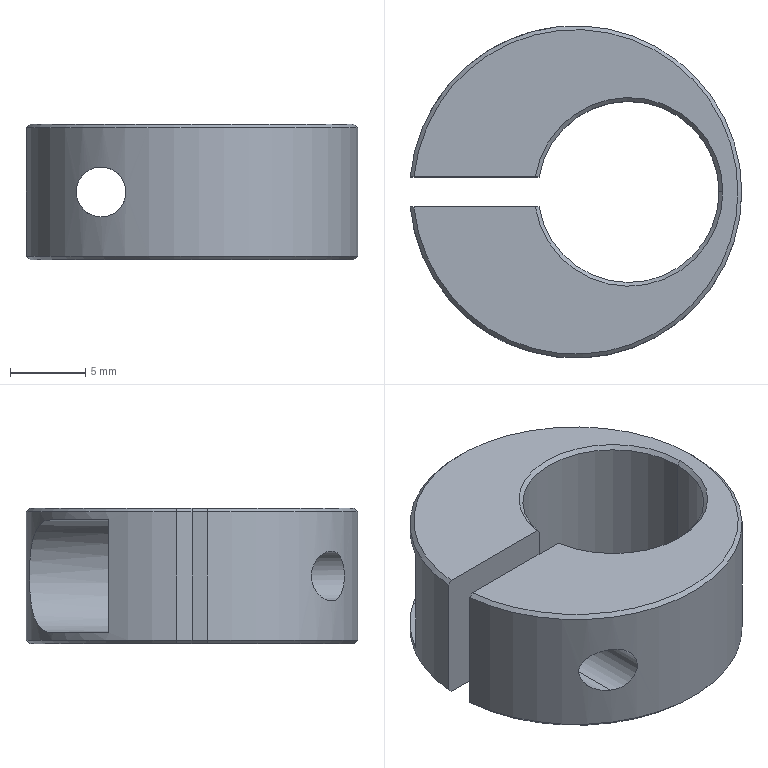Part | NX | features BREP 1 | 1 solid | 21 faces | box 21.954 x 22 x 9 mm | volume 1945 mm3 | cylinder 8 | plane 7 | cone 6 | commonest cylinder face diameters 3.3 x2 4.5 x2 12 x2 7.5 x1 22 x1
STEP:
#1=CARTESIAN_POINT('',(9.5,0.,8.75));
#2=VERTEX_POINT('',#1);
#3=CARTESIAN_POINT('',(9.75,0.,9.));
#4=VERTEX_POINT('',#3);
#5=CARTESIAN_POINT('',(9.5,0.,8.75));
#6=DIRECTION('',(0.7071,0.,0.7071));
#7=VECTOR('',#6,1000.);
#8=LINE('',#5,#7);
#9=EDGE_CURVE('',#2,#4,#8,.T.);
#10=ORIENTED_EDGE('',*,*,#9,.F.);
#11=CARTESIAN_POINT('',(-2.416,-1.,8.75));
#12=VERTEX_POINT('',#11);
#13=CARTESIAN_POINT('',(3.5,0.,8.75));
#14=DIRECTION('',(0.,0.,1.));
#15=DIRECTION('',(1.,0.,0.));
#16=AXIS2_PLACEMENT_3D('',#13,#14,#15);
#17=CIRCLE('',#16,6.);
#18=EDGE_CURVE('',#12,#2,#17,.T.);
#19=ORIENTED_EDGE('',*,*,#18,.F.);
#20=CARTESIAN_POINT('',(-2.669,-1.,9.));
#21=VERTEX_POINT('',#20);
#22=CARTESIAN_POINT('',(-2.669,-1.,9.));
#23=CARTESIAN_POINT('',(-2.585,-1.,8.917));
#24=CARTESIAN_POINT('',(-2.501,-1.,8.833));
#25=CARTESIAN_POINT('',(-2.416,-1.,8.75));
#26=B_SPLINE_CURVE_WITH_KNOTS('',3,(#22,#23,#24,#25),.UNSPECIFIED.,.F.,.F.,(4,4),(0.,0.000356),.UNSPECIFIED.);
#27=EDGE_CURVE('',#21,#12,#26,.T.);
#28=ORIENTED_EDGE('',*,*,#27,.F.);
#29=CARTESIAN_POINT('',(3.5,0.,9.));
#30=DIRECTION('',(0.,0.,-1.));
#31=DIRECTION('',(1.,0.,0.));
#32=AXIS2_PLACEMENT_3D('',#29,#30,#31);
#33=CIRCLE('',#32,6.25);
#34=EDGE_CURVE('',#4,#21,#33,.T.);
#35=ORIENTED_EDGE('',*,*,#34,.F.);
#36=EDGE_LOOP('',(#10,#19,#28,#35));
#37=FACE_BOUND('',#36,.T.);
#38=CARTESIAN_POINT('',(3.5,0.,8.75));
#39=DIRECTION('',(0.,0.,1.));
#40=DIRECTION('',(1.,0.,0.));
#41=AXIS2_PLACEMENT_3D('',#38,#39,#40);
#42=CONICAL_SURFACE('',#41,6.,0.7854);
#43=ADVANCED_FACE('',(#37),#42,.F.);
#44=CARTESIAN_POINT('',(-10.954,-1.,8.75));
#45=VERTEX_POINT('',#44);
#46=CARTESIAN_POINT('',(-10.703,-1.,9.));
#47=VERTEX_POINT('',#46);
#48=CARTESIAN_POINT('',(-10.954,-1.,8.75));
#49=CARTESIAN_POINT('',(-10.871,-1.,8.833));
#50=CARTESIAN_POINT('',(-10.787,-1.,8.917));
#51=CARTESIAN_POINT('',(-10.703,-1.,9.));
#52=B_SPLINE_CURVE_WITH_KNOTS('',3,(#48,#49,#50,#51),.UNSPECIFIED.,.F.,.F.,(4,4),(0.,0.0003543),.UNSPECIFIED.);
#53=EDGE_CURVE('',#45,#47,#52,.T.);
#54=ORIENTED_EDGE('',*,*,#53,.F.);
#55=CARTESIAN_POINT('',(-10.954,1.,8.75));
#56=VERTEX_POINT('',#55);
#57=CARTESIAN_POINT('',(0.,0.,8.75));
#58=DIRECTION('',(0.,0.,-1.));
#59=DIRECTION('',(1.,0.,0.));
#60=AXIS2_PLACEMENT_3D('',#57,#58,#59);
#61=CIRCLE('',#60,11.);
#62=EDGE_CURVE('',#56,#45,#61,.T.);
#63=ORIENTED_EDGE('',*,*,#62,.F.);
#64=CARTESIAN_POINT('',(-10.703,1.,9.));
#65=VERTEX_POINT('',#64);
#66=CARTESIAN_POINT('',(-10.703,1.,9.));
#67=CARTESIAN_POINT('',(-10.787,1.,8.917));
#68=CARTESIAN_POINT('',(-10.871,1.,8.833));
#69=CARTESIAN_POINT('',(-10.954,1.,8.75));
#70=B_SPLINE_CURVE_WITH_KNOTS('',3,(#66,#67,#68,#69),.UNSPECIFIED.,.F.,.F.,(4,4),(0.,0.0003543),.UNSPECIFIED.);
#71=EDGE_CURVE('',#65,#56,#70,.T.);
#72=ORIENTED_EDGE('',*,*,#71,.F.);
#73=CARTESIAN_POINT('',(0.,0.,9.));
#74=DIRECTION('',(0.,0.,1.));
#75=DIRECTION('',(1.,0.,0.));
#76=AXIS2_PLACEMENT_3D('',#73,#74,#75);
#77=CIRCLE('',#76,10.75);
#78=EDGE_CURVE('',#47,#65,#77,.T.);
#79=ORIENTED_EDGE('',*,*,#78,.F.);
#80=EDGE_LOOP('',(#54,#63,#72,#79));
#81=FACE_BOUND('',#80,.T.);
#82=CARTESIAN_POINT('',(0.,0.,9.));
#83=DIRECTION('',(0.,0.,-1.));
#84=DIRECTION('',(-1.,0.,0.));
#85=AXIS2_PLACEMENT_3D('',#82,#83,#84);
#86=CONICAL_SURFACE('',#85,10.75,0.7854);
#87=ADVANCED_FACE('',(#81),#86,.T.);
#88=CARTESIAN_POINT('',(-2.669,1.,0.));
#89=VERTEX_POINT('',#88);
#90=CARTESIAN_POINT('',(-2.416,1.,0.25));
#91=VERTEX_POINT('',#90);
#92=CARTESIAN_POINT('',(-2.669,1.,0.));
#93=CARTESIAN_POINT('',(-2.585,1.,0.08336));
#94=CARTESIAN_POINT('',(-2.501,1.,0.1667));
#95=CARTESIAN_POINT('',(-2.416,1.,0.25));
#96=B_SPLINE_CURVE_WITH_KNOTS('',3,(#92,#93,#94,#95),.UNSPECIFIED.,.F.,.F.,(4,4),(0.,0.000356),.UNSPECIFIED.);
#97=EDGE_CURVE('',#89,#91,#96,.T.);
#98=ORIENTED_EDGE('',*,*,#97,.F.);
#99=CARTESIAN_POINT('',(-2.669,-1.,0.));
#100=VERTEX_POINT('',#99);
#101=CARTESIAN_POINT('',(3.5,0.,0.));
#102=DIRECTION('',(0.,0.,1.));
#103=DIRECTION('',(1.,0.,0.));
#104=AXIS2_PLACEMENT_3D('',#101,#102,#103);
#105=CIRCLE('',#104,6.25);
#106=EDGE_CURVE('',#100,#89,#105,.T.);
#107=ORIENTED_EDGE('',*,*,#106,.F.);
#108=CARTESIAN_POINT('',(-2.416,-1.,0.25));
#109=VERTEX_POINT('',#108);
#110=CARTESIAN_POINT('',(-2.416,-1.,0.25));
#111=CARTESIAN_POINT('',(-2.501,-1.,0.1667));
#112=CARTESIAN_POINT('',(-2.585,-1.,0.08336));
#113=CARTESIAN_POINT('',(-2.669,-1.,0.));
#114=B_SPLINE_CURVE_WITH_KNOTS('',3,(#110,#111,#112,#113),.UNSPECIFIED.,.F.,.F.,(4,4),(0.,0.000356),.UNSPECIFIED.);
#115=EDGE_CURVE('',#109,#100,#114,.T.);
#116=ORIENTED_EDGE('',*,*,#115,.F.);
#117=CARTESIAN_POINT('',(9.5,0.,0.25));
#118=VERTEX_POINT('',#117);
#119=CARTESIAN_POINT('',(3.5,0.,0.25));
#120=DIRECTION('',(0.,0.,-1.));
#121=DIRECTION('',(1.,0.,0.));
#122=AXIS2_PLACEMENT_3D('',#119,#120,#121);
#123=CIRCLE('',#122,6.);
#124=EDGE_CURVE('',#118,#109,#123,.T.);
#125=ORIENTED_EDGE('',*,*,#124,.F.);
#126=CARTESIAN_POINT('',(3.5,0.,0.25));
#127=DIRECTION('',(0.,0.,-1.));
#128=DIRECTION('',(1.,0.,0.));
#129=AXIS2_PLACEMENT_3D('',#126,#127,#128);
#130=CIRCLE('',#129,6.);
#131=EDGE_CURVE('',#91,#118,#130,.T.);
#132=ORIENTED_EDGE('',*,*,#131,.F.);
#133=EDGE_LOOP('',(#98,#107,#116,#125,#132));
#134=FACE_BOUND('',#133,.T.);
#135=CARTESIAN_POINT('',(3.5,0.,0.25));
#136=DIRECTION('',(0.,0.,-1.));
#137=DIRECTION('',(-1.,0.,0.));
#138=AXIS2_PLACEMENT_3D('',#135,#136,#137);
#139=CONICAL_SURFACE('',#138,6.,0.7854);
#140=ADVANCED_FACE('',(#134),#139,.F.);
#141=CARTESIAN_POINT('',(10.75,0.,0.));
#142=VERTEX_POINT('',#141);
#143=CARTESIAN_POINT('',(11.,0.,0.25));
#144=VERTEX_POINT('',#143);
#145=CARTESIAN_POINT('',(11.,0.,0.25));
#146=DIRECTION('',(0.7071,0.,0.7071));
#147=VECTOR('',#146,1000.);
#148=LINE('',#145,#147);
#149=EDGE_CURVE('',#142,#144,#148,.T.);
#150=ORIENTED_EDGE('',*,*,#149,.F.);
#151=CARTESIAN_POINT('',(-10.703,1.,0.));
#152=VERTEX_POINT('',#151);
#153=CARTESIAN_POINT('',(0.,0.,0.));
#154=DIRECTION('',(0.,0.,-1.));
#155=DIRECTION('',(1.,0.,0.));
#156=AXIS2_PLACEMENT_3D('',#153,#154,#155);
#157=CIRCLE('',#156,10.75);
#158=EDGE_CURVE('',#152,#142,#157,.T.);
#159=ORIENTED_EDGE('',*,*,#158,.F.);
#160=CARTESIAN_POINT('',(-10.954,1.,0.25));
#161=VERTEX_POINT('',#160);
#162=CARTESIAN_POINT('',(-10.954,1.,0.25));
#163=CARTESIAN_POINT('',(-10.871,1.,0.1667));
#164=CARTESIAN_POINT('',(-10.787,1.,0.08333));
#165=CARTESIAN_POINT('',(-10.703,1.,0.));
#166=B_SPLINE_CURVE_WITH_KNOTS('',3,(#162,#163,#164,#165),.UNSPECIFIED.,.F.,.F.,(4,4),(0.,0.0003543),.UNSPECIFIED.);
#167=EDGE_CURVE('',#161,#152,#166,.T.);
#168=ORIENTED_EDGE('',*,*,#167,.F.);
#169=CARTESIAN_POINT('',(0.,0.,0.25));
#170=DIRECTION('',(0.,0.,1.));
#171=DIRECTION('',(1.,0.,0.));
#172=AXIS2_PLACEMENT_3D('',#169,#170,#171);
#173=CIRCLE('',#172,11.);
#174=EDGE_CURVE('',#144,#161,#173,.T.);
#175=ORIENTED_EDGE('',*,*,#174,.F.);
#176=EDGE_LOOP('',(#150,#159,#168,#175));
#177=FACE_BOUND('',#176,.T.);
#178=CARTESIAN_POINT('',(0.,0.,0.25));
#179=DIRECTION('',(0.,0.,1.));
#180=DIRECTION('',(1.,0.,0.));
#181=AXIS2_PLACEMENT_3D('',#178,#179,#180);
#182=CONICAL_SURFACE('',#181,11.,0.7854);
#183=ADVANCED_FACE('',(#177),#182,.T.);
#184=CARTESIAN_POINT('',(-6.,-1.,2.85));
#185=VERTEX_POINT('',#184);
#186=CARTESIAN_POINT('',(-6.,-9.22,2.85));
#187=VERTEX_POINT('',#186);
#188=CARTESIAN_POINT('',(-6.,-1.,2.85));
#189=DIRECTION('',(0.,1.,0.));
#190=VECTOR('',#189,1000.);
#191=LINE('',#188,#190);
#192=EDGE_CURVE('',#185,#187,#191,.F.);
#193=ORIENTED_EDGE('',*,*,#192,.T.);
#194=CARTESIAN_POINT('',(-6.,-9.22,6.15));
#195=VERTEX_POINT('',#194);
#196=CARTESIAN_POINT('',(-6.,-9.22,2.85));
#197=CARTESIAN_POINT('',(-5.573,-9.497,2.85));
#198=CARTESIAN_POINT('',(-4.796,-9.917,3.131));
#199=CARTESIAN_POINT('',(-4.125,-10.197,4.506));
#200=CARTESIAN_POINT('',(-4.804,-9.914,5.873));
#201=CARTESIAN_POINT('',(-5.574,-9.496,6.15));
#202=CARTESIAN_POINT('',(-6.,-9.22,6.15));
#203=B_SPLINE_CURVE_WITH_KNOTS('',3,(#196,#197,#198,#199,#200,#201,#202),.UNSPECIFIED.,.F.,.F.,(4,1,1,1,4),(0.,0.25,0.5,0.75,1.),.UNSPECIFIED.);
#204=EDGE_CURVE('',#195,#187,#203,.F.);
#205=ORIENTED_EDGE('',*,*,#204,.F.);
#206=CARTESIAN_POINT('',(-6.,-1.,6.15));
#207=VERTEX_POINT('',#206);
#208=CARTESIAN_POINT('',(-6.,-1.,6.15));
#209=DIRECTION('',(0.,1.,0.));
#210=VECTOR('',#209,1000.);
#211=LINE('',#208,#210);
#212=EDGE_CURVE('',#207,#195,#211,.F.);
#213=ORIENTED_EDGE('',*,*,#212,.F.);
#214=CARTESIAN_POINT('',(-6.,-1.,4.5));
#215=DIRECTION('',(0.,1.,0.));
#216=DIRECTION('',(0.,0.,1.));
#217=AXIS2_PLACEMENT_3D('',#214,#215,#216);
#218=CIRCLE('',#217,1.65);
#219=EDGE_CURVE('',#207,#185,#218,.T.);
#220=ORIENTED_EDGE('',*,*,#219,.T.);
#221=EDGE_LOOP('',(#193,#205,#213,#220));
#222=FACE_BOUND('',#221,.T.);
#223=CARTESIAN_POINT('',(-6.,-1.,4.5));
#224=DIRECTION('',(0.,1.,0.));
#225=DIRECTION('',(0.,0.,1.));
#226=AXIS2_PLACEMENT_3D('',#223,#224,#225);
#227=CYLINDRICAL_SURFACE('',#226,1.65);
#228=ADVANCED_FACE('',(#222),#227,.F.);
#229=CARTESIAN_POINT('',(-6.,9.22,0.75));
#230=VERTEX_POINT('',#229);
#231=CARTESIAN_POINT('',(-9.526,5.5,0.75));
#232=VERTEX_POINT('',#231);
#233=CARTESIAN_POINT('',(0.,0.,0.75));
#234=DIRECTION('',(0.,0.,1.));
#235=DIRECTION('',(1.,0.,0.));
#236=AXIS2_PLACEMENT_3D('',#233,#234,#235);
#237=CIRCLE('',#236,11.);
#238=EDGE_CURVE('',#230,#232,#237,.T.);
#239=ORIENTED_EDGE('',*,*,#238,.T.);
#240=CARTESIAN_POINT('',(-6.,5.5,0.75));
#241=VERTEX_POINT('',#240);
#242=CARTESIAN_POINT('',(-6.,5.5,0.75));
#243=DIRECTION('',(-1.,0.,0.));
#244=VECTOR('',#243,1000.);
#245=LINE('',#242,#244);
#246=EDGE_CURVE('',#241,#232,#245,.T.);
#247=ORIENTED_EDGE('',*,*,#246,.F.);
#248=CARTESIAN_POINT('',(-6.,11.001,0.75));
#249=DIRECTION('',(0.,1.,0.));
#250=VECTOR('',#249,1000.);
#251=LINE('',#248,#250);
#252=EDGE_CURVE('',#241,#230,#251,.T.);
#253=ORIENTED_EDGE('',*,*,#252,.T.);
#254=EDGE_LOOP('',(#239,#247,#253));
#255=FACE_BOUND('',#254,.T.);
#256=CARTESIAN_POINT('',(-6.,10.,0.75));
#257=DIRECTION('',(0.,0.,1.));
#258=DIRECTION('',(1.,0.,0.));
#259=AXIS2_PLACEMENT_3D('',#256,#257,#258);
#260=PLANE('',#259);
#261=ADVANCED_FACE('',(#255),#260,.T.);
#262=CARTESIAN_POINT('',(-9.526,5.5,8.25));
#263=VERTEX_POINT('',#262);
#264=CARTESIAN_POINT('',(-6.,9.22,8.25));
#265=VERTEX_POINT('',#264);
#266=CARTESIAN_POINT('',(0.,0.,8.25));
#267=DIRECTION('',(0.,0.,-1.));
#268=DIRECTION('',(-1.,0.,0.));
#269=AXIS2_PLACEMENT_3D('',#266,#267,#268);
#270=CIRCLE('',#269,11.);
#271=EDGE_CURVE('',#263,#265,#270,.T.);
#272=ORIENTED_EDGE('',*,*,#271,.T.);
#273=CARTESIAN_POINT('',(-6.,5.5,8.25));
#274=VERTEX_POINT('',#273);
#275=CARTESIAN_POINT('',(-6.,11.001,8.25));
#276=DIRECTION('',(0.,-1.,0.));
#277=VECTOR('',#276,1000.);
#278=LINE('',#275,#277);
#279=EDGE_CURVE('',#265,#274,#278,.T.);
#280=ORIENTED_EDGE('',*,*,#279,.T.);
#281=CARTESIAN_POINT('',(-6.,5.5,8.25));
#282=DIRECTION('',(1.,0.,0.));
#283=VECTOR('',#282,1000.);
#284=LINE('',#281,#283);
#285=EDGE_CURVE('',#263,#274,#284,.T.);
#286=ORIENTED_EDGE('',*,*,#285,.F.);
#287=EDGE_LOOP('',(#272,#280,#286));
#288=FACE_BOUND('',#287,.T.);
#289=CARTESIAN_POINT('',(-6.,10.,8.25));
#290=DIRECTION('',(0.,0.,-1.));
#291=DIRECTION('',(-1.,0.,0.));
#292=AXIS2_PLACEMENT_3D('',#289,#290,#291);
#293=PLANE('',#292);
#294=ADVANCED_FACE('',(#288),#293,.T.);
#295=CARTESIAN_POINT('',(-9.526,5.5,9.));
#296=DIRECTION('',(0.,0.,1.));
#297=VECTOR('',#296,1000.);
#298=LINE('',#295,#297);
#299=EDGE_CURVE('',#232,#263,#298,.T.);
#300=ORIENTED_EDGE('',*,*,#299,.T.);
#301=ORIENTED_EDGE('',*,*,#285,.T.);
#302=CARTESIAN_POINT('',(-6.,5.5,4.5));
#303=DIRECTION('',(0.,-1.,0.));
#304=DIRECTION('',(0.,0.,-1.));
#305=AXIS2_PLACEMENT_3D('',#302,#303,#304);
#306=CIRCLE('',#305,3.75);
#307=EDGE_CURVE('',#241,#274,#306,.T.);
#308=ORIENTED_EDGE('',*,*,#307,.F.);
#309=ORIENTED_EDGE('',*,*,#246,.T.);
#310=EDGE_LOOP('',(#300,#301,#308,#309));
#311=FACE_BOUND('',#310,.T.);
#312=CARTESIAN_POINT('',(-6.,5.5,2.25));
#313=VERTEX_POINT('',#312);
#314=CARTESIAN_POINT('',(-6.,5.5,6.75));
#315=VERTEX_POINT('',#314);
#316=CARTESIAN_POINT('',(-6.,5.5,4.5));
#317=DIRECTION('',(0.,1.,0.));
#318=DIRECTION('',(0.,0.,-1.));
#319=AXIS2_PLACEMENT_3D('',#316,#317,#318);
#320=CIRCLE('',#319,2.25);
#321=EDGE_CURVE('',#313,#315,#320,.T.);
#322=ORIENTED_EDGE('',*,*,#321,.F.);
#323=CARTESIAN_POINT('',(-6.,5.5,4.5));
#324=DIRECTION('',(0.,1.,0.));
#325=DIRECTION('',(0.,0.,-1.));
#326=AXIS2_PLACEMENT_3D('',#323,#324,#325);
#327=CIRCLE('',#326,2.25);
#328=EDGE_CURVE('',#315,#313,#327,.T.);
#329=ORIENTED_EDGE('',*,*,#328,.F.);
#330=EDGE_LOOP('',(#322,#329));
#331=FACE_BOUND('',#330,.T.);
#332=CARTESIAN_POINT('',(-6.,5.5,4.5));
#333=DIRECTION('',(0.,-1.,0.));
#334=DIRECTION('',(0.,0.,-1.));
#335=AXIS2_PLACEMENT_3D('',#332,#333,#334);
#336=PLANE('',#335);
#337=ADVANCED_FACE('',(#311,#331),#336,.F.);
#338=CARTESIAN_POINT('',(-6.,1.,6.75));
#339=VERTEX_POINT('',#338);
#340=CARTESIAN_POINT('',(-6.,5.5,6.75));
#341=DIRECTION('',(0.,-1.,0.));
#342=VECTOR('',#341,1000.);
#343=LINE('',#340,#342);
#344=EDGE_CURVE('',#315,#339,#343,.T.);
#345=ORIENTED_EDGE('',*,*,#344,.F.);
#346=ORIENTED_EDGE('',*,*,#328,.T.);
#347=CARTESIAN_POINT('',(-6.,1.,2.25));
#348=VERTEX_POINT('',#347);
#349=CARTESIAN_POINT('',(-6.,5.5,2.25));
#350=DIRECTION('',(0.,-1.,0.));
#351=VECTOR('',#350,1000.);
#352=LINE('',#349,#351);
#353=EDGE_CURVE('',#313,#348,#352,.T.);
#354=ORIENTED_EDGE('',*,*,#353,.T.);
#355=CARTESIAN_POINT('',(-6.,1.,4.5));
#356=DIRECTION('',(0.,-1.,0.));
#357=DIRECTION('',(0.,0.,-1.));
#358=AXIS2_PLACEMENT_3D('',#355,#356,#357);
#359=CIRCLE('',#358,2.25);
#360=EDGE_CURVE('',#348,#339,#359,.T.);
#361=ORIENTED_EDGE('',*,*,#360,.T.);
#362=EDGE_LOOP('',(#345,#346,#354,#361));
#363=FACE_BOUND('',#362,.T.);
#364=CARTESIAN_POINT('',(-6.,5.5,4.5));
#365=DIRECTION('',(0.,-1.,0.));
#366=DIRECTION('',(0.,0.,-1.));
#367=AXIS2_PLACEMENT_3D('',#364,#365,#366);
#368=CYLINDRICAL_SURFACE('',#367,2.25);
#369=ADVANCED_FACE('',(#363),#368,.F.);
#370=CARTESIAN_POINT('',(-10.703,-1.,0.));
#371=VERTEX_POINT('',#370);
#372=CARTESIAN_POINT('',(-19.584,-1.,0.));
#373=DIRECTION('',(-1.,0.,0.));
#374=VECTOR('',#373,1000.);
#375=LINE('',#372,#374);
#376=EDGE_CURVE('',#100,#371,#375,.T.);
#377=ORIENTED_EDGE('',*,*,#376,.T.);
#378=CARTESIAN_POINT('',(-10.954,-1.,0.25));
#379=VERTEX_POINT('',#378);
#380=CARTESIAN_POINT('',(-10.703,-1.,0.));
#381=CARTESIAN_POINT('',(-10.787,-1.,0.08333));
#382=CARTESIAN_POINT('',(-10.871,-1.,0.1667));
#383=CARTESIAN_POINT('',(-10.954,-1.,0.25));
#384=B_SPLINE_CURVE_WITH_KNOTS('',3,(#380,#381,#382,#383),.UNSPECIFIED.,.F.,.F.,(4,4),(0.,0.0003543),.UNSPECIFIED.);
#385=EDGE_CURVE('',#371,#379,#384,.T.);
#386=ORIENTED_EDGE('',*,*,#385,.T.);
#387=CARTESIAN_POINT('',(-10.954,-1.,9.));
#388=DIRECTION('',(0.,0.,1.));
#389=VECTOR('',#388,1000.);
#390=LINE('',#387,#389);
#391=EDGE_CURVE('',#379,#45,#390,.T.);
#392=ORIENTED_EDGE('',*,*,#391,.T.);
#393=ORIENTED_EDGE('',*,*,#53,.T.);
#394=CARTESIAN_POINT('',(-19.584,-1.,9.));
#395=DIRECTION('',(1.,0.,0.));
#396=VECTOR('',#395,1000.);
#397=LINE('',#394,#396);
#398=EDGE_CURVE('',#47,#21,#397,.T.);
#399=ORIENTED_EDGE('',*,*,#398,.T.);
#400=ORIENTED_EDGE('',*,*,#27,.T.);
#401=CARTESIAN_POINT('',(-2.416,-1.,-0.001));
#402=DIRECTION('',(0.,0.,-1.));
#403=VECTOR('',#402,1000.);
#404=LINE('',#401,#403);
#405=EDGE_CURVE('',#12,#109,#404,.T.);
#406=ORIENTED_EDGE('',*,*,#405,.T.);
#407=ORIENTED_EDGE('',*,*,#115,.T.);
#408=EDGE_LOOP('',(#377,#386,#392,#393,#399,#400,#406,#407));
#409=FACE_BOUND('',#408,.T.);
#410=ORIENTED_EDGE('',*,*,#219,.F.);
#411=CARTESIAN_POINT('',(-6.,-1.,4.5));
#412=DIRECTION('',(0.,1.,0.));
#413=DIRECTION('',(0.,0.,1.));
#414=AXIS2_PLACEMENT_3D('',#411,#412,#413);
#415=CIRCLE('',#414,1.65);
#416=EDGE_CURVE('',#185,#207,#415,.T.);
#417=ORIENTED_EDGE('',*,*,#416,.F.);
#418=EDGE_LOOP('',(#410,#417));
#419=FACE_BOUND('',#418,.T.);
#420=CARTESIAN_POINT('',(-19.584,-1.,-0.001));
#421=DIRECTION('',(0.,-1.,0.));
#422=DIRECTION('',(0.,0.,-1.));
#423=AXIS2_PLACEMENT_3D('',#420,#421,#422);
#424=PLANE('',#423);
#425=ADVANCED_FACE('',(#409,#419),#424,.F.);
#426=CARTESIAN_POINT('',(-10.954,1.,9.));
#427=DIRECTION('',(0.,0.,-1.));
#428=VECTOR('',#427,1000.);
#429=LINE('',#426,#428);
#430=EDGE_CURVE('',#56,#161,#429,.T.);
#431=ORIENTED_EDGE('',*,*,#430,.T.);
#432=ORIENTED_EDGE('',*,*,#167,.T.);
#433=CARTESIAN_POINT('',(-19.584,1.,0.));
#434=DIRECTION('',(1.,0.,0.));
#435=VECTOR('',#434,1000.);
#436=LINE('',#433,#435);
#437=EDGE_CURVE('',#152,#89,#436,.T.);
#438=ORIENTED_EDGE('',*,*,#437,.T.);
#439=ORIENTED_EDGE('',*,*,#97,.T.);
#440=CARTESIAN_POINT('',(-2.416,1.,8.75));
#441=VERTEX_POINT('',#440);
#442=CARTESIAN_POINT('',(-2.416,1.,-0.001));
#443=DIRECTION('',(0.,0.,1.));
#444=VECTOR('',#443,1000.);
#445=LINE('',#442,#444);
#446=EDGE_CURVE('',#91,#441,#445,.T.);
#447=ORIENTED_EDGE('',*,*,#446,.T.);
#448=CARTESIAN_POINT('',(-2.669,1.,9.));
#449=VERTEX_POINT('',#448);
#450=CARTESIAN_POINT('',(-2.416,1.,8.75));
#451=CARTESIAN_POINT('',(-2.501,1.,8.833));
#452=CARTESIAN_POINT('',(-2.585,1.,8.917));
#453=CARTESIAN_POINT('',(-2.669,1.,9.));
#454=B_SPLINE_CURVE_WITH_KNOTS('',3,(#450,#451,#452,#453),.UNSPECIFIED.,.F.,.F.,(4,4),(0.,0.000356),.UNSPECIFIED.);
#455=EDGE_CURVE('',#441,#449,#454,.T.);
#456=ORIENTED_EDGE('',*,*,#455,.T.);
#457=CARTESIAN_POINT('',(-19.584,1.,9.));
#458=DIRECTION('',(-1.,0.,0.));
#459=VECTOR('',#458,1000.);
#460=LINE('',#457,#459);
#461=EDGE_CURVE('',#449,#65,#460,.T.);
#462=ORIENTED_EDGE('',*,*,#461,.T.);
#463=ORIENTED_EDGE('',*,*,#71,.T.);
#464=EDGE_LOOP('',(#431,#432,#438,#439,#447,#456,#462,#463));
#465=FACE_BOUND('',#464,.T.);
#466=ORIENTED_EDGE('',*,*,#360,.F.);
#467=CARTESIAN_POINT('',(-6.,1.,4.5));
#468=DIRECTION('',(0.,-1.,0.));
#469=DIRECTION('',(0.,0.,-1.));
#470=AXIS2_PLACEMENT_3D('',#467,#468,#469);
#471=CIRCLE('',#470,2.25);
#472=EDGE_CURVE('',#339,#348,#471,.T.);
#473=ORIENTED_EDGE('',*,*,#472,.F.);
#474=EDGE_LOOP('',(#466,#473));
#475=FACE_BOUND('',#474,.T.);
#476=CARTESIAN_POINT('',(-19.584,1.,-0.001));
#477=DIRECTION('',(0.,1.,0.));
#478=DIRECTION('',(0.,0.,1.));
#479=AXIS2_PLACEMENT_3D('',#476,#477,#478);
#480=PLANE('',#479);
#481=ADVANCED_FACE('',(#465,#475),#480,.F.);
#482=CARTESIAN_POINT('',(9.5,0.,-0.001));
#483=DIRECTION('',(0.,0.,1.));
#484=VECTOR('',#483,1000.);
#485=LINE('',#482,#484);
#486=EDGE_CURVE('',#118,#2,#485,.T.);
#487=ORIENTED_EDGE('',*,*,#486,.F.);
#488=ORIENTED_EDGE('',*,*,#124,.T.);
#489=ORIENTED_EDGE('',*,*,#405,.F.);
#490=ORIENTED_EDGE('',*,*,#18,.T.);
#491=EDGE_LOOP('',(#487,#488,#489,#490));
#492=FACE_BOUND('',#491,.T.);
#493=CARTESIAN_POINT('',(3.5,0.,-0.001));
#494=DIRECTION('',(0.,0.,1.));
#495=DIRECTION('',(1.,0.,0.));
#496=AXIS2_PLACEMENT_3D('',#493,#494,#495);
#497=CYLINDRICAL_SURFACE('',#496,6.);
#498=ADVANCED_FACE('',(#492),#497,.F.);
#499=ORIENTED_EDGE('',*,*,#437,.F.);
#500=ORIENTED_EDGE('',*,*,#158,.T.);
#501=CARTESIAN_POINT('',(0.,0.,0.));
#502=DIRECTION('',(0.,0.,-1.));
#503=DIRECTION('',(1.,0.,0.));
#504=AXIS2_PLACEMENT_3D('',#501,#502,#503);
#505=CIRCLE('',#504,10.75);
#506=EDGE_CURVE('',#142,#371,#505,.T.);
#507=ORIENTED_EDGE('',*,*,#506,.T.);
#508=ORIENTED_EDGE('',*,*,#376,.F.);
#509=ORIENTED_EDGE('',*,*,#106,.T.);
#510=EDGE_LOOP('',(#499,#500,#507,#508,#509));
#511=FACE_BOUND('',#510,.T.);
#512=CARTESIAN_POINT('',(0.,0.,0.));
#513=DIRECTION('',(0.,0.,1.));
#514=DIRECTION('',(1.,0.,0.));
#515=AXIS2_PLACEMENT_3D('',#512,#513,#514);
#516=PLANE('',#515);
#517=ADVANCED_FACE('',(#511),#516,.F.);
#518=ORIENTED_EDGE('',*,*,#398,.F.);
#519=ORIENTED_EDGE('',*,*,#78,.T.);
#520=ORIENTED_EDGE('',*,*,#461,.F.);
#521=CARTESIAN_POINT('',(3.5,0.,9.));
#522=DIRECTION('',(0.,0.,-1.));
#523=DIRECTION('',(1.,0.,0.));
#524=AXIS2_PLACEMENT_3D('',#521,#522,#523);
#525=CIRCLE('',#524,6.25);
#526=EDGE_CURVE('',#449,#4,#525,.T.);
#527=ORIENTED_EDGE('',*,*,#526,.T.);
#528=ORIENTED_EDGE('',*,*,#34,.T.);
#529=EDGE_LOOP('',(#518,#519,#520,#527,#528));
#530=FACE_BOUND('',#529,.T.);
#531=CARTESIAN_POINT('',(0.,0.,9.));
#532=DIRECTION('',(0.,0.,1.));
#533=DIRECTION('',(1.,0.,0.));
#534=AXIS2_PLACEMENT_3D('',#531,#532,#533);
#535=PLANE('',#534);
#536=ADVANCED_FACE('',(#530),#535,.T.);
#537=ORIENTED_EDGE('',*,*,#279,.F.);
#538=CARTESIAN_POINT('',(-6.,9.22,8.25));
#539=CARTESIAN_POINT('',(-5.55,9.513,8.25));
#540=CARTESIAN_POINT('',(-4.674,9.995,8.11));
#541=CARTESIAN_POINT('',(-3.357,10.497,7.286));
#542=CARTESIAN_POINT('',(-2.541,10.708,6.19));
#543=CARTESIAN_POINT('',(-2.105,10.797,4.506));
#544=CARTESIAN_POINT('',(-2.538,10.708,2.817));
#545=CARTESIAN_POINT('',(-3.352,10.498,1.718));
#546=CARTESIAN_POINT('',(-4.673,9.995,0.89));
#547=CARTESIAN_POINT('',(-5.549,9.513,0.75));
#548=CARTESIAN_POINT('',(-6.,9.22,0.75));
#549=B_SPLINE_CURVE_WITH_KNOTS('',3,(#538,#539,#540,#541,#542,#543,#544,#545,#546,#547,#548),.UNSPECIFIED.,.F.,.F.,(4,1,1,1,1,1,1,1,4),(0.,0.125,0.25,0.375,0.5,0.625,0.75,0.875,1.),.UNSPECIFIED.);
#550=EDGE_CURVE('',#265,#230,#549,.T.);
#551=ORIENTED_EDGE('',*,*,#550,.T.);
#552=ORIENTED_EDGE('',*,*,#252,.F.);
#553=ORIENTED_EDGE('',*,*,#307,.T.);
#554=EDGE_LOOP('',(#537,#551,#552,#553));
#555=FACE_BOUND('',#554,.T.);
#556=CARTESIAN_POINT('',(-6.,11.001,4.5));
#557=DIRECTION('',(0.,-1.,0.));
#558=DIRECTION('',(0.,0.,-1.));
#559=AXIS2_PLACEMENT_3D('',#556,#557,#558);
#560=CYLINDRICAL_SURFACE('',#559,3.75);
#561=ADVANCED_FACE('',(#555),#560,.F.);
#562=ORIENTED_EDGE('',*,*,#271,.F.);
#563=ORIENTED_EDGE('',*,*,#299,.F.);
#564=ORIENTED_EDGE('',*,*,#238,.F.);
#565=ORIENTED_EDGE('',*,*,#550,.F.);
#566=EDGE_LOOP('',(#562,#563,#564,#565));
#567=FACE_BOUND('',#566,.T.);
#568=ORIENTED_EDGE('',*,*,#391,.F.);
#569=CARTESIAN_POINT('',(0.,0.,0.25));
#570=DIRECTION('',(0.,0.,1.));
#571=DIRECTION('',(1.,0.,0.));
#572=AXIS2_PLACEMENT_3D('',#569,#570,#571);
#573=CIRCLE('',#572,11.);
#574=EDGE_CURVE('',#379,#144,#573,.T.);
#575=ORIENTED_EDGE('',*,*,#574,.T.);
#576=ORIENTED_EDGE('',*,*,#174,.T.);
#577=ORIENTED_EDGE('',*,*,#430,.F.);
#578=ORIENTED_EDGE('',*,*,#62,.T.);
#579=EDGE_LOOP('',(#568,#575,#576,#577,#578));
#580=FACE_BOUND('',#579,.T.);
#581=ORIENTED_EDGE('',*,*,#204,.T.);
#582=CARTESIAN_POINT('',(-6.,-9.22,2.85));
#583=CARTESIAN_POINT('',(-6.41,-8.953,2.85));
#584=CARTESIAN_POINT('',(-6.998,-8.504,3.074));
#585=CARTESIAN_POINT('',(-7.532,-8.02,3.766));
#586=CARTESIAN_POINT('',(-7.709,-7.847,4.5));
#587=CARTESIAN_POINT('',(-7.533,-8.019,5.233));
#588=CARTESIAN_POINT('',(-6.998,-8.505,5.926));
#589=CARTESIAN_POINT('',(-6.41,-8.953,6.15));
#590=CARTESIAN_POINT('',(-6.,-9.22,6.15));
#591=B_SPLINE_CURVE_WITH_KNOTS('',3,(#582,#583,#584,#585,#586,#587,#588,#589,#590),.UNSPECIFIED.,.F.,.F.,(4,1,1,1,1,1,4),(0.,0.25,0.375,0.5,0.625,0.75,1.),.UNSPECIFIED.);
#592=EDGE_CURVE('',#187,#195,#591,.T.);
#593=ORIENTED_EDGE('',*,*,#592,.T.);
#594=EDGE_LOOP('',(#581,#593));
#595=FACE_BOUND('',#594,.T.);
#596=CARTESIAN_POINT('',(0.,0.,9.));
#597=DIRECTION('',(0.,0.,-1.));
#598=DIRECTION('',(-1.,0.,0.));
#599=AXIS2_PLACEMENT_3D('',#596,#597,#598);
#600=CYLINDRICAL_SURFACE('',#599,11.);
#601=ADVANCED_FACE('',(#567,#580,#595),#600,.T.);
#602=ORIENTED_EDGE('',*,*,#131,.T.);
#603=ORIENTED_EDGE('',*,*,#486,.T.);
#604=CARTESIAN_POINT('',(3.5,0.,8.75));
#605=DIRECTION('',(0.,0.,1.));
#606=DIRECTION('',(1.,0.,0.));
#607=AXIS2_PLACEMENT_3D('',#604,#605,#606);
#608=CIRCLE('',#607,6.);
#609=EDGE_CURVE('',#2,#441,#608,.T.);
#610=ORIENTED_EDGE('',*,*,#609,.T.);
#611=ORIENTED_EDGE('',*,*,#446,.F.);
#612=EDGE_LOOP('',(#602,#603,#610,#611));
#613=FACE_BOUND('',#612,.T.);
#614=CARTESIAN_POINT('',(3.5,0.,-0.001));
#615=DIRECTION('',(0.,0.,1.));
#616=DIRECTION('',(1.,0.,0.));
#617=AXIS2_PLACEMENT_3D('',#614,#615,#616);
#618=CYLINDRICAL_SURFACE('',#617,6.);
#619=ADVANCED_FACE('',(#613),#618,.F.);
#620=ORIENTED_EDGE('',*,*,#321,.T.);
#621=ORIENTED_EDGE('',*,*,#344,.T.);
#622=ORIENTED_EDGE('',*,*,#472,.T.);
#623=ORIENTED_EDGE('',*,*,#353,.F.);
#624=EDGE_LOOP('',(#620,#621,#622,#623));
#625=FACE_BOUND('',#624,.T.);
#626=CARTESIAN_POINT('',(-6.,5.5,4.5));
#627=DIRECTION('',(0.,-1.,0.));
#628=DIRECTION('',(0.,0.,-1.));
#629=AXIS2_PLACEMENT_3D('',#626,#627,#628);
#630=CYLINDRICAL_SURFACE('',#629,2.25);
#631=ADVANCED_FACE('',(#625),#630,.F.);
#632=ORIENTED_EDGE('',*,*,#592,.F.);
#633=ORIENTED_EDGE('',*,*,#192,.F.);
#634=ORIENTED_EDGE('',*,*,#416,.T.);
#635=ORIENTED_EDGE('',*,*,#212,.T.);
#636=EDGE_LOOP('',(#632,#633,#634,#635));
#637=FACE_BOUND('',#636,.T.);
#638=CARTESIAN_POINT('',(-6.,-1.,4.5));
#639=DIRECTION('',(0.,1.,0.));
#640=DIRECTION('',(0.,0.,1.));
#641=AXIS2_PLACEMENT_3D('',#638,#639,#640);
#642=CYLINDRICAL_SURFACE('',#641,1.65);
#643=ADVANCED_FACE('',(#637),#642,.F.);
#644=ORIENTED_EDGE('',*,*,#506,.F.);
#645=ORIENTED_EDGE('',*,*,#149,.T.);
#646=ORIENTED_EDGE('',*,*,#574,.F.);
#647=ORIENTED_EDGE('',*,*,#385,.F.);
#648=EDGE_LOOP('',(#644,#645,#646,#647));
#649=FACE_BOUND('',#648,.T.);
#650=CARTESIAN_POINT('',(0.,0.,0.25));
#651=DIRECTION('',(0.,0.,1.));
#652=DIRECTION('',(1.,0.,0.));
#653=AXIS2_PLACEMENT_3D('',#650,#651,#652);
#654=CONICAL_SURFACE('',#653,11.,0.7854);
#655=ADVANCED_FACE('',(#649),#654,.T.);
#656=ORIENTED_EDGE('',*,*,#609,.F.);
#657=ORIENTED_EDGE('',*,*,#9,.T.);
#658=ORIENTED_EDGE('',*,*,#526,.F.);
#659=ORIENTED_EDGE('',*,*,#455,.F.);
#660=EDGE_LOOP('',(#656,#657,#658,#659));
#661=FACE_BOUND('',#660,.T.);
#662=CARTESIAN_POINT('',(3.5,0.,8.75));
#663=DIRECTION('',(0.,0.,1.));
#664=DIRECTION('',(1.,0.,0.));
#665=AXIS2_PLACEMENT_3D('',#662,#663,#664);
#666=CONICAL_SURFACE('',#665,6.,0.7854);
#667=ADVANCED_FACE('',(#661),#666,.F.);
#668=CLOSED_SHELL('',(#43,#87,#140,#183,#228,#261,#294,#337,#369,#425,#481,#498,#517,#536,#561,#601,#619,#631,#643,#655,#667));
#669=MANIFOLD_SOLID_BREP('',#668);
#670=(LENGTH_UNIT()NAMED_UNIT(*)SI_UNIT(.MILLI.,.METRE.));
#671=UNCERTAINTY_MEASURE_WITH_UNIT(LENGTH_MEASURE(0.0508),#670,'','');
#672=(NAMED_UNIT(*)PLANE_ANGLE_UNIT()SI_UNIT($,.RADIAN.));
#673=(NAMED_UNIT(*)SI_UNIT($,.STERADIAN.)SOLID_ANGLE_UNIT());
#674=(GEOMETRIC_REPRESENTATION_CONTEXT(3)GLOBAL_UNCERTAINTY_ASSIGNED_CONTEXT((#671))GLOBAL_UNIT_ASSIGNED_CONTEXT((#670,#672,#673))REPRESENTATION_CONTEXT('',''));
#675=ADVANCED_BREP_SHAPE_REPRESENTATION('',(#669),#674);